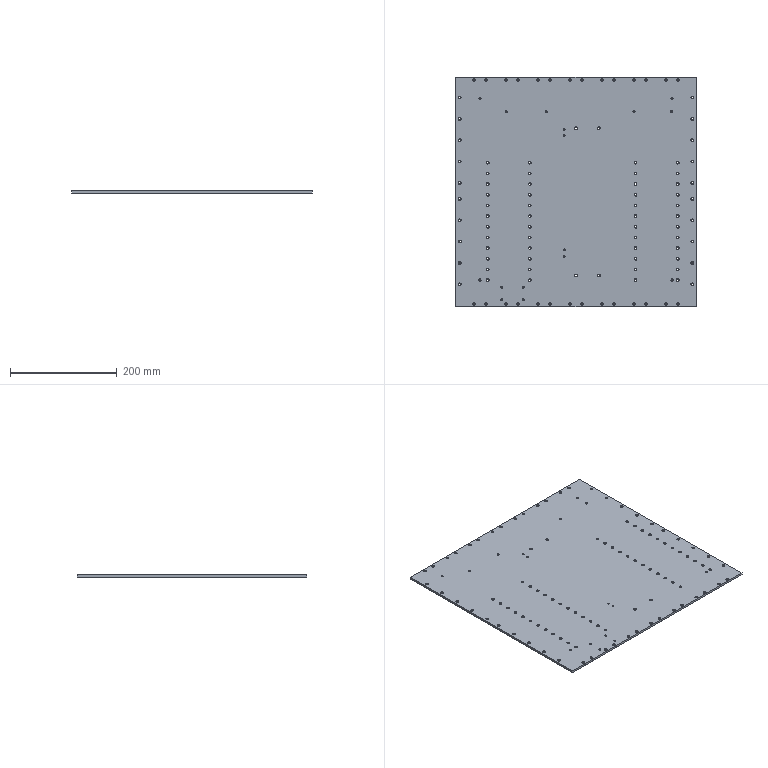Part | STEP file | Chassis bottom plate | 1 solid | 354 faces | box 450 x 430 x 4 mm | volume 764514 mm3 | cone 232 | cylinder 116 | plane 6 | commonest cylinder face diameters 4.3 x100 3.3 x8 2.7 x4 3.2 x4